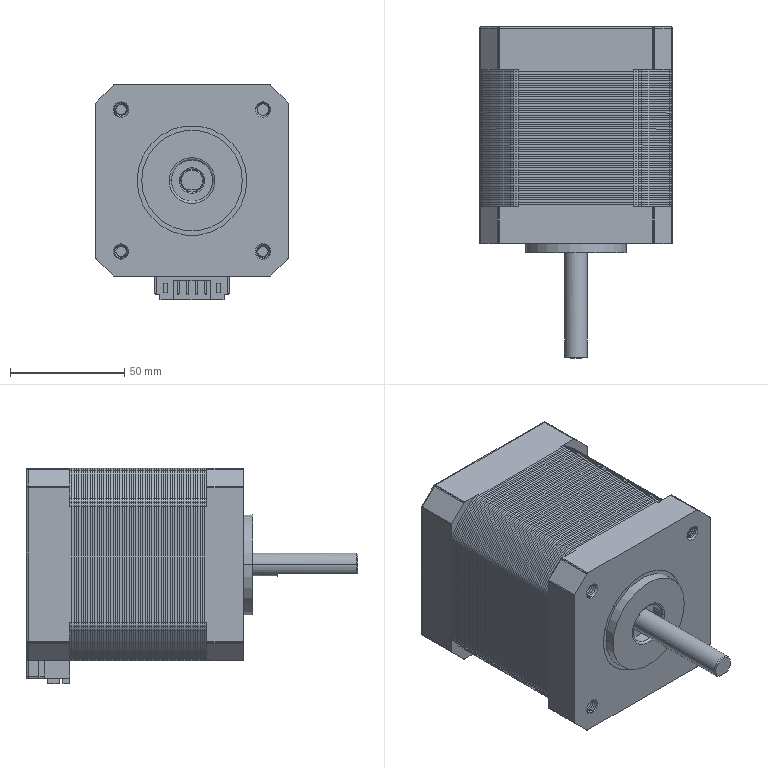Part | STEP file | 1 solid | 2054 faces | box 84 x 145 x 94 mm | volume 649991 mm3 | cylinder 1462 | plane 448 | cone 40 | torus 40 | spline 40 | sphere 24 | commonest cylinder face diameters 12 x960 100 x240 6.172 x96 2 x64 1.166 x48 5.058 x26